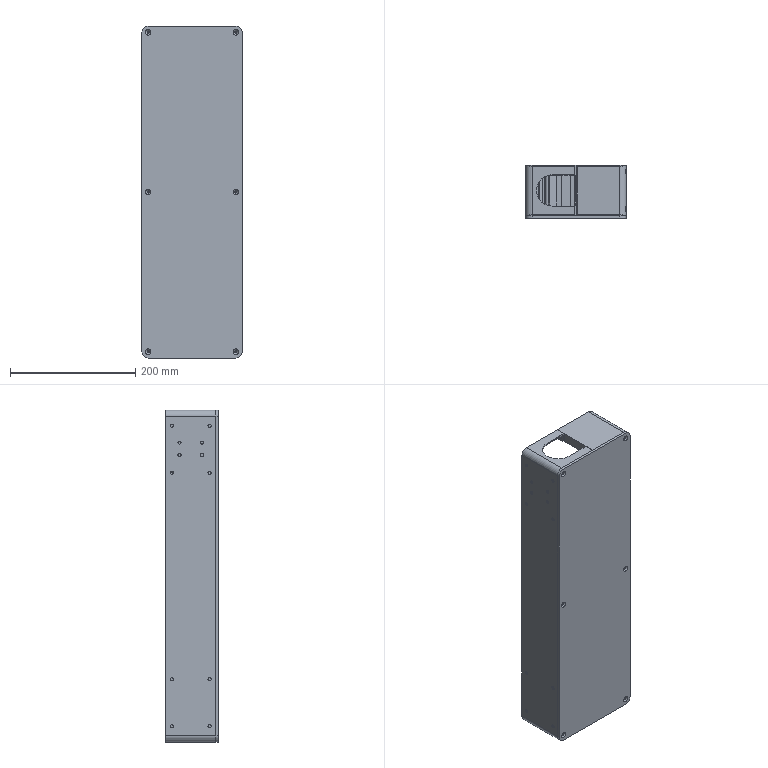Part | NX | 3 solids | 1199 faces | box 160 x 84 x 530 mm | volume 843813 mm3 | plane 909 | cylinder 280 | cone 10 | commonest cylinder face diameters 1 x44 28 x44 28.4 x40 10 x32 2 x22 0.4 x20